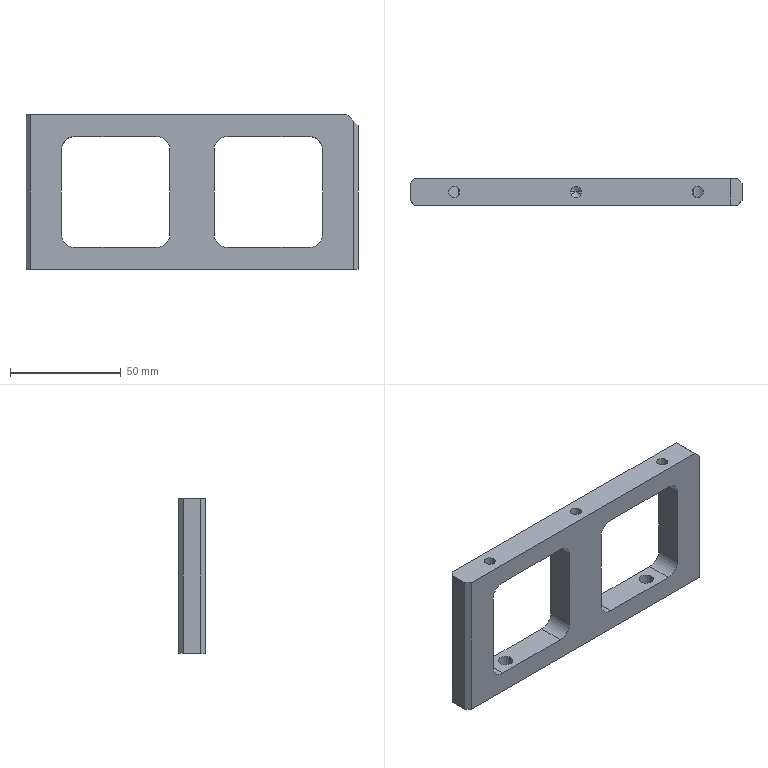Part | STEP file | QA-AD17 | 1 solid | 39 faces | box 150 x 12 x 70 mm | volume 65829 mm3 | plane 19 | cylinder 18 | cone 2 | commonest cylinder face diameters 12 x8 5 x6 6.5 x4